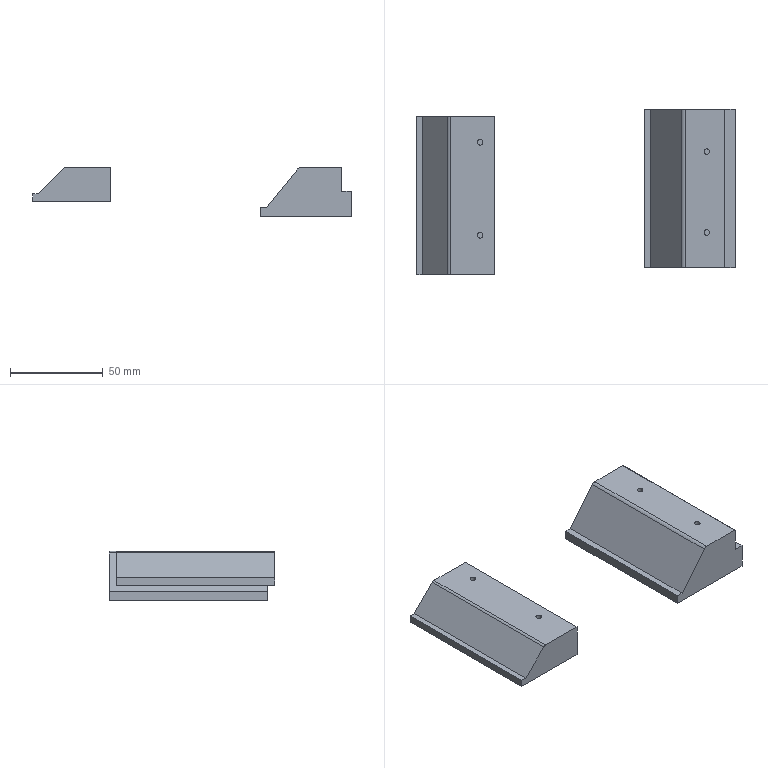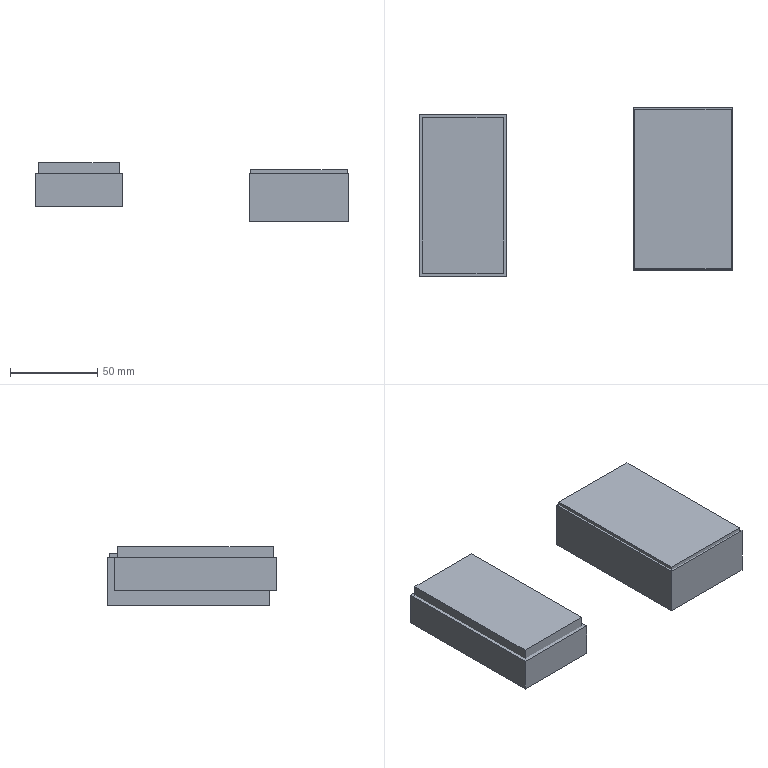CAM job | NX | 3-axis milling | part box 171.319 x 88.841 x 26.598 mm | stock box 179.319 x 96.841 x 33.598 mm
Tools:
number,name,description,diameter,corner_radius,flute_length,length,flutes
19,D80,Milling Tool-5 Parameters,80.0,0.0,50.0,75.0,2
15,D10,Milling Tool-5 Parameters,10.0,0.0,50.0,75.0,2
14,D10JING,Milling Tool-5 Parameters,10.0,0.0,50.0,75.0,2
16,D6R0.5,Milling Tool-5 Parameters,6.0,0.5,50.0,75.0,2
17,D2,Milling Tool-5 Parameters,2.0,0.0,50.0,75.0,2
1,D6A45,Milling Tool-5 Parameters,6.0,0.0,50.0,75.0,2
Operations:
program,operation,operation_type,tool,method,geometry_group,spindle_rpm,surface_speed,feed_per_tooth,feed_cut,feed_plunge,cut_length_mm,path_length_mm,cut_time_min,machine_time_min
1,FLOOR_WALL_COPY,VolumeBased25DMillingOperation,D80,METHOD,A,6500.0,1633.0,0.1154,1500.0,100.0,189.0,243.0,0.126,0.1314
1,ADAPTIVE_MILLING,CavityMilling,D10,METHOD,A,9500.0,298.0,0.1579,3000.0,1000.0,6087.183,8092.435,2.055,2.256
1,ZLEVEL_PROFILE_COPY_1_COPY_COPY_1,ZLevelMilling,D10JING,METHOD,A,9500.0,298.0,0.0632,1200.0,1000.0,292.754,387.358,0.2446,0.254
1,FLOOR_WALL_1,VolumeBased25DMillingOperation,D10JING,METHOD,A,9500.0,298.0,0.0658,1250.0,100.0,107.0,189.604,0.0856,0.0939
1,ZLEVEL_PROFILE,ZLevelMilling,D6R0.5,METHOD,A,9500.0,179.0,0.1579,3000.0,1000.0,18643.577,18714.884,6.216,6.224
1,HOLE_MILLING,CylinderMilling,D2,METHOD,A,9500.0,59.0,0.0526,1000.0,100.0,192.175,371.174,0.1922,0.2101
1,PLANAR_MILL_COPY_COPY_COPY_COPY_COPY_COPY_1_COPY_1,PlanarMilling,D6A45,METHOD,A,9500.0,179.0,0.0658,1250.0,100.0,162.257,457.368,0.1298,0.1593
1,刀补17,CylinderMilling,D2,METHOD,A,9500.0,59.0,0.0526,1000.0,100.0,41.442,220.441,0.0414,0.0593
2,FLOOR_WALL_COPY_COPY,VolumeBased25DMillingOperation,D80,METHOD,B,6500.0,1633.0,0.1154,1500.0,100.0,1295.0,2705.002,0.8633,1.004
2,PLANAR_MILL_COPY_COPY_COPY_COPY_COPY_COPY_1_COPY_1_COPY,PlanarMilling,D6A45,METHOD,B,9500.0,179.0,0.0658,1250.0,100.0,266.194,325.194,0.213,0.2189
11,FLOOR_WALL_COPY_COPY_1,VolumeBased25DMillingOperation,D80,METHOD,C,6500.0,1633.0,0.1154,1500.0,100.0,189.0,243.0,0.126,0.1314
11,ADAPTIVE_MILLING_COPY,CavityMilling,D10,METHOD,C,9500.0,298.0,0.1579,3000.0,1000.0,6427.093,9879.885,2.184,2.53
11,ZLEVEL_PROFILE_COPY_1_COPY_COPY_1_COPY,ZLevelMilling,D10JING,METHOD,C,9500.0,298.0,0.0632,1200.0,1000.0,306.754,417.951,0.2562,0.2673
11,FLOOR_WALL_1_COPY,VolumeBased25DMillingOperation,D10JING,METHOD,C,9500.0,298.0,0.0658,1250.0,100.0,309.154,599.24,0.2473,0.2763
11,ZLEVEL_PROFILE_COPY,ZLevelMilling,D6R0.5,METHOD,C,9500.0,179.0,0.1579,3000.0,1000.0,25437.818,25516.424,8.481,8.489
11,ZLEVEL_PROFILE_COPY_COPY,ZLevelMilling,D6R0.5,METHOD,C,9500.0,179.0,0.1579,3000.0,1000.0,1399.289,1457.302,0.4684,0.4742
11,HOLE_MILLING_COPY,CylinderMilling,D2,METHOD,C,9500.0,59.0,0.0526,1000.0,100.0,192.175,364.674,0.1922,0.2094
11,PLANAR_MILL_COPY_COPY_COPY_COPY_COPY_COPY_1_COPY_1_COPY_1,PlanarMilling,D6A45,METHOD,C,9500.0,179.0,0.0658,1250.0,100.0,73.153,466.041,0.0585,0.0978
11,PLANAR_MILL_COPY_COPY_COPY_COPY_COPY_COPY_1_COPY_1_COPY_1_COPY,PlanarMilling,D6A45,METHOD,C,9500.0,179.0,0.0658,1250.0,100.0,97.646,182.645,0.0781,0.0866
11,刀补17_COPY,CylinderMilling,D2,METHOD,C,9500.0,59.0,0.0526,1000.0,100.0,41.442,213.941,0.0414,0.0587
22,FLOOR_WALL_COPY_COPY_COPY,VolumeBased25DMillingOperation,D80,METHOD,D,6500.0,1633.0,0.1154,1500.0,100.0,561.0,1079.001,0.374,0.4258
22,PLANAR_MILL_COPY_COPY_COPY_COPY_COPY_COPY_1_COPY_1_COPY_COPY,PlanarMilling,D6A45,METHOD,D,9500.0,179.0,0.0658,1250.0,100.0,280.194,339.194,0.2242,0.2301